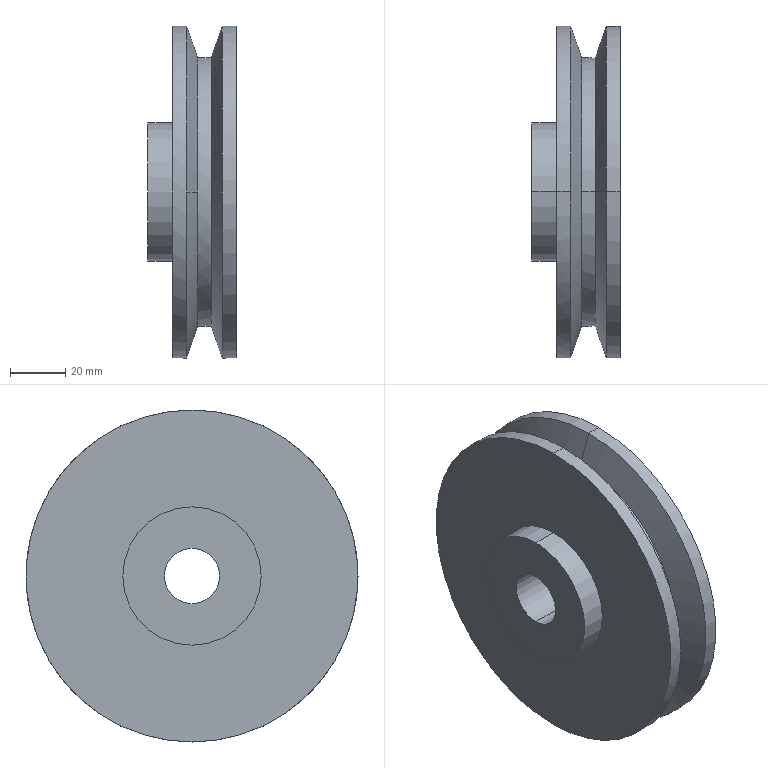Part | SolidWorks | features BaseBody 1, ICE 1 | 1 solid | 17 faces | box 32 x 120 x 120 mm | volume 232249 mm3 | cylinder 10 | cone 4 | plane 3 | commonest cylinder face diameters 120 x4 20 x2 50 x2 97.1 x2
STEP:
#1=CARTESIAN_POINT('',(21.,0.,-10.));
#2=VERTEX_POINT('',#1);
#3=CARTESIAN_POINT('',(21.,0.,10.));
#4=VERTEX_POINT('',#3);
#5=CARTESIAN_POINT('',(21.,0.,0.));
#6=DIRECTION('',(-1.,0.,0.));
#7=DIRECTION('',(0.,0.,1.));
#8=AXIS2_PLACEMENT_3D('',#5,#6,#7);
#9=CIRCLE('',#8,10.);
#10=EDGE_CURVE('',#2,#4,#9,.T.);
#11=ORIENTED_EDGE('',*,*,#10,.F.);
#12=CARTESIAN_POINT('',(-11.,0.,-10.));
#13=VERTEX_POINT('',#12);
#14=CARTESIAN_POINT('',(21.,0.,-10.));
#15=DIRECTION('',(-1.,0.,0.));
#16=VECTOR('',#15,1000.);
#17=LINE('',#14,#16);
#18=EDGE_CURVE('',#2,#13,#17,.T.);
#19=ORIENTED_EDGE('',*,*,#18,.T.);
#20=CARTESIAN_POINT('',(-11.,0.,10.));
#21=VERTEX_POINT('',#20);
#22=CARTESIAN_POINT('',(-11.,0.,0.));
#23=DIRECTION('',(-1.,0.,0.));
#24=DIRECTION('',(0.,0.,1.));
#25=AXIS2_PLACEMENT_3D('',#22,#23,#24);
#26=CIRCLE('',#25,10.);
#27=EDGE_CURVE('',#13,#21,#26,.T.);
#28=ORIENTED_EDGE('',*,*,#27,.T.);
#29=CARTESIAN_POINT('',(21.,0.,10.));
#30=DIRECTION('',(-1.,0.,0.));
#31=VECTOR('',#30,1000.);
#32=LINE('',#29,#31);
#33=EDGE_CURVE('',#4,#21,#32,.T.);
#34=ORIENTED_EDGE('',*,*,#33,.F.);
#35=EDGE_LOOP('',(#11,#19,#28,#34));
#36=FACE_OUTER_BOUND('',#35,.T.);
#37=CARTESIAN_POINT('',(21.,0.,0.));
#38=DIRECTION('',(-1.,0.,0.));
#39=DIRECTION('',(0.,0.,1.));
#40=AXIS2_PLACEMENT_3D('',#37,#38,#39);
#41=CYLINDRICAL_SURFACE('',#40,10.);
#42=ADVANCED_FACE('',(#36),#41,.F.);
#43=CARTESIAN_POINT('',(15.947,0.,-60.));
#44=VERTEX_POINT('',#43);
#45=CARTESIAN_POINT('',(15.947,0.,60.));
#46=VERTEX_POINT('',#45);
#47=CARTESIAN_POINT('',(15.947,0.,0.));
#48=DIRECTION('',(1.,0.,0.));
#49=DIRECTION('',(0.,0.,-1.));
#50=AXIS2_PLACEMENT_3D('',#47,#48,#49);
#51=CIRCLE('',#50,60.);
#52=EDGE_CURVE('',#44,#46,#51,.T.);
#53=ORIENTED_EDGE('',*,*,#52,.T.);
#54=CARTESIAN_POINT('',(21.,0.,60.));
#55=VERTEX_POINT('',#54);
#56=CARTESIAN_POINT('',(0.,0.,60.));
#57=DIRECTION('',(1.,0.,0.));
#58=VECTOR('',#57,1000.);
#59=LINE('',#56,#58);
#60=EDGE_CURVE('',#46,#55,#59,.T.);
#61=ORIENTED_EDGE('',*,*,#60,.T.);
#62=CARTESIAN_POINT('',(21.,0.,-60.));
#63=VERTEX_POINT('',#62);
#64=CARTESIAN_POINT('',(21.,0.,0.));
#65=DIRECTION('',(1.,0.,0.));
#66=DIRECTION('',(0.,0.,-1.));
#67=AXIS2_PLACEMENT_3D('',#64,#65,#66);
#68=CIRCLE('',#67,60.);
#69=EDGE_CURVE('',#63,#55,#68,.T.);
#70=ORIENTED_EDGE('',*,*,#69,.F.);
#71=CARTESIAN_POINT('',(0.,0.,-60.));
#72=DIRECTION('',(1.,0.,0.));
#73=VECTOR('',#72,1000.);
#74=LINE('',#71,#73);
#75=EDGE_CURVE('',#44,#63,#74,.T.);
#76=ORIENTED_EDGE('',*,*,#75,.F.);
#77=EDGE_LOOP('',(#53,#61,#70,#76));
#78=FACE_OUTER_BOUND('',#77,.T.);
#79=CARTESIAN_POINT('',(0.,0.,0.));
#80=DIRECTION('',(1.,0.,0.));
#81=DIRECTION('',(0.,0.,-1.));
#82=AXIS2_PLACEMENT_3D('',#79,#80,#81);
#83=CYLINDRICAL_SURFACE('',#82,60.);
#84=ADVANCED_FACE('',(#78),#83,.T.);
#85=CARTESIAN_POINT('',(12.004,0.,-48.55));
#86=VERTEX_POINT('',#85);
#87=CARTESIAN_POINT('',(12.004,0.,48.55));
#88=VERTEX_POINT('',#87);
#89=CARTESIAN_POINT('',(12.004,0.,0.));
#90=DIRECTION('',(1.,0.,0.));
#91=DIRECTION('',(0.,0.,-1.));
#92=AXIS2_PLACEMENT_3D('',#89,#90,#91);
#93=CIRCLE('',#92,48.55);
#94=EDGE_CURVE('',#86,#88,#93,.T.);
#95=ORIENTED_EDGE('',*,*,#94,.T.);
#96=CARTESIAN_POINT('',(15.947,0.,60.));
#97=DIRECTION('',(0.3256,0.,0.9455));
#98=VECTOR('',#97,1000.);
#99=LINE('',#96,#98);
#100=EDGE_CURVE('',#88,#46,#99,.T.);
#101=ORIENTED_EDGE('',*,*,#100,.T.);
#102=ORIENTED_EDGE('',*,*,#52,.F.);
#103=CARTESIAN_POINT('',(15.947,0.,-60.));
#104=DIRECTION('',(0.3256,0.,-0.9455));
#105=VECTOR('',#104,1000.);
#106=LINE('',#103,#105);
#107=EDGE_CURVE('',#86,#44,#106,.T.);
#108=ORIENTED_EDGE('',*,*,#107,.F.);
#109=EDGE_LOOP('',(#95,#101,#102,#108));
#110=FACE_OUTER_BOUND('',#109,.T.);
#111=CARTESIAN_POINT('',(15.947,0.,0.));
#112=DIRECTION('',(1.,0.,0.));
#113=DIRECTION('',(0.,0.,-1.));
#114=AXIS2_PLACEMENT_3D('',#111,#112,#113);
#115=CONICAL_SURFACE('',#114,60.,1.239);
#116=ADVANCED_FACE('',(#110),#115,.T.);
#117=CARTESIAN_POINT('',(-11.,0.,25.));
#118=VERTEX_POINT('',#117);
#119=CARTESIAN_POINT('',(-11.,0.,-25.));
#120=VERTEX_POINT('',#119);
#121=CARTESIAN_POINT('',(-11.,0.,0.));
#122=DIRECTION('',(-1.,0.,0.));
#123=DIRECTION('',(0.,0.,-1.));
#124=AXIS2_PLACEMENT_3D('',#121,#122,#123);
#125=CIRCLE('',#124,25.);
#126=EDGE_CURVE('',#118,#120,#125,.T.);
#127=ORIENTED_EDGE('',*,*,#126,.F.);
#128=CARTESIAN_POINT('',(-2.,0.,25.));
#129=VERTEX_POINT('',#128);
#130=CARTESIAN_POINT('',(0.,0.,25.));
#131=DIRECTION('',(1.,0.,0.));
#132=VECTOR('',#131,1000.);
#133=LINE('',#130,#132);
#134=EDGE_CURVE('',#118,#129,#133,.T.);
#135=ORIENTED_EDGE('',*,*,#134,.T.);
#136=CARTESIAN_POINT('',(-2.,0.,-25.));
#137=VERTEX_POINT('',#136);
#138=CARTESIAN_POINT('',(-2.,0.,0.));
#139=DIRECTION('',(-1.,0.,0.));
#140=DIRECTION('',(0.,0.,-1.));
#141=AXIS2_PLACEMENT_3D('',#138,#139,#140);
#142=CIRCLE('',#141,25.);
#143=EDGE_CURVE('',#129,#137,#142,.T.);
#144=ORIENTED_EDGE('',*,*,#143,.T.);
#145=CARTESIAN_POINT('',(0.,0.,-25.));
#146=DIRECTION('',(1.,0.,0.));
#147=VECTOR('',#146,1000.);
#148=LINE('',#145,#147);
#149=EDGE_CURVE('',#120,#137,#148,.T.);
#150=ORIENTED_EDGE('',*,*,#149,.F.);
#151=EDGE_LOOP('',(#127,#135,#144,#150));
#152=FACE_OUTER_BOUND('',#151,.T.);
#153=CARTESIAN_POINT('',(0.,0.,0.));
#154=DIRECTION('',(1.,0.,0.));
#155=DIRECTION('',(0.,0.,-1.));
#156=AXIS2_PLACEMENT_3D('',#153,#154,#155);
#157=CYLINDRICAL_SURFACE('',#156,25.);
#158=ADVANCED_FACE('',(#152),#157,.T.);
#159=ORIENTED_EDGE('',*,*,#94,.F.);
#160=CARTESIAN_POINT('',(6.996,0.,-48.55));
#161=VERTEX_POINT('',#160);
#162=CARTESIAN_POINT('',(0.,0.,-48.55));
#163=DIRECTION('',(-1.,0.,0.));
#164=VECTOR('',#163,1000.);
#165=LINE('',#162,#164);
#166=EDGE_CURVE('',#86,#161,#165,.T.);
#167=ORIENTED_EDGE('',*,*,#166,.T.);
#168=CARTESIAN_POINT('',(6.996,48.55,0.));
#169=VERTEX_POINT('',#168);
#170=CARTESIAN_POINT('',(6.996,0.,0.));
#171=DIRECTION('',(1.,0.,0.));
#172=DIRECTION('',(0.,0.,1.));
#173=AXIS2_PLACEMENT_3D('',#170,#171,#172);
#174=CIRCLE('',#173,48.55);
#175=EDGE_CURVE('',#161,#169,#174,.T.);
#176=ORIENTED_EDGE('',*,*,#175,.T.);
#177=CARTESIAN_POINT('',(6.996,0.,48.55));
#178=VERTEX_POINT('',#177);
#179=CARTESIAN_POINT('',(6.996,0.,0.));
#180=DIRECTION('',(1.,0.,0.));
#181=DIRECTION('',(0.,0.,1.));
#182=AXIS2_PLACEMENT_3D('',#179,#180,#181);
#183=CIRCLE('',#182,48.55);
#184=EDGE_CURVE('',#169,#178,#183,.T.);
#185=ORIENTED_EDGE('',*,*,#184,.T.);
#186=CARTESIAN_POINT('',(0.,0.,48.55));
#187=DIRECTION('',(-1.,0.,0.));
#188=VECTOR('',#187,1000.);
#189=LINE('',#186,#188);
#190=EDGE_CURVE('',#88,#178,#189,.T.);
#191=ORIENTED_EDGE('',*,*,#190,.F.);
#192=EDGE_LOOP('',(#159,#167,#176,#185,#191));
#193=FACE_OUTER_BOUND('',#192,.T.);
#194=CARTESIAN_POINT('',(0.,0.,0.));
#195=DIRECTION('',(-1.,0.,0.));
#196=DIRECTION('',(0.,0.,1.));
#197=AXIS2_PLACEMENT_3D('',#194,#195,#196);
#198=CYLINDRICAL_SURFACE('',#197,48.55);
#199=ADVANCED_FACE('',(#193),#198,.T.);
#200=ORIENTED_EDGE('',*,*,#184,.F.);
#201=CARTESIAN_POINT('',(3.053,60.,0.));
#202=VERTEX_POINT('',#201);
#203=CARTESIAN_POINT('',(3.053,60.,0.));
#204=DIRECTION('',(-0.3256,0.9455,0.));
#205=VECTOR('',#204,1000.);
#206=LINE('',#203,#205);
#207=EDGE_CURVE('',#169,#202,#206,.T.);
#208=ORIENTED_EDGE('',*,*,#207,.T.);
#209=CARTESIAN_POINT('',(3.053,0.,60.));
#210=VERTEX_POINT('',#209);
#211=CARTESIAN_POINT('',(3.053,0.,0.));
#212=DIRECTION('',(1.,0.,0.));
#213=DIRECTION('',(0.,0.,1.));
#214=AXIS2_PLACEMENT_3D('',#211,#212,#213);
#215=CIRCLE('',#214,60.);
#216=EDGE_CURVE('',#202,#210,#215,.T.);
#217=ORIENTED_EDGE('',*,*,#216,.T.);
#218=CARTESIAN_POINT('',(3.053,-60.,0.));
#219=VERTEX_POINT('',#218);
#220=CARTESIAN_POINT('',(3.053,0.,0.));
#221=DIRECTION('',(1.,0.,0.));
#222=DIRECTION('',(0.,0.,1.));
#223=AXIS2_PLACEMENT_3D('',#220,#221,#222);
#224=CIRCLE('',#223,60.);
#225=EDGE_CURVE('',#210,#219,#224,.T.);
#226=ORIENTED_EDGE('',*,*,#225,.T.);
#227=CARTESIAN_POINT('',(6.996,-48.55,0.));
#228=VERTEX_POINT('',#227);
#229=CARTESIAN_POINT('',(3.053,-60.,0.));
#230=DIRECTION('',(-0.3256,-0.9455,0.));
#231=VECTOR('',#230,1000.);
#232=LINE('',#229,#231);
#233=EDGE_CURVE('',#228,#219,#232,.T.);
#234=ORIENTED_EDGE('',*,*,#233,.F.);
#235=CARTESIAN_POINT('',(6.996,0.,0.));
#236=DIRECTION('',(1.,0.,0.));
#237=DIRECTION('',(0.,0.,1.));
#238=AXIS2_PLACEMENT_3D('',#235,#236,#237);
#239=CIRCLE('',#238,48.55);
#240=EDGE_CURVE('',#178,#228,#239,.T.);
#241=ORIENTED_EDGE('',*,*,#240,.F.);
#242=EDGE_LOOP('',(#200,#208,#217,#226,#234,#241));
#243=FACE_OUTER_BOUND('',#242,.T.);
#244=CARTESIAN_POINT('',(3.053,0.,0.));
#245=DIRECTION('',(-1.,0.,0.));
#246=DIRECTION('',(0.,-1.,0.));
#247=AXIS2_PLACEMENT_3D('',#244,#245,#246);
#248=CONICAL_SURFACE('',#247,60.,1.239);
#249=ADVANCED_FACE('',(#243),#248,.T.);
#250=CARTESIAN_POINT('',(-2.,0.,60.));
#251=VERTEX_POINT('',#250);
#252=CARTESIAN_POINT('',(-2.,0.,-60.));
#253=VERTEX_POINT('',#252);
#254=CARTESIAN_POINT('',(-2.,0.,0.));
#255=DIRECTION('',(-1.,0.,0.));
#256=DIRECTION('',(0.,0.,-1.));
#257=AXIS2_PLACEMENT_3D('',#254,#255,#256);
#258=CIRCLE('',#257,60.);
#259=EDGE_CURVE('',#251,#253,#258,.T.);
#260=ORIENTED_EDGE('',*,*,#259,.F.);
#261=CARTESIAN_POINT('',(0.,0.,60.));
#262=DIRECTION('',(1.,0.,0.));
#263=VECTOR('',#262,1000.);
#264=LINE('',#261,#263);
#265=EDGE_CURVE('',#251,#210,#264,.T.);
#266=ORIENTED_EDGE('',*,*,#265,.T.);
#267=ORIENTED_EDGE('',*,*,#216,.F.);
#268=CARTESIAN_POINT('',(3.053,0.,-60.));
#269=VERTEX_POINT('',#268);
#270=CARTESIAN_POINT('',(3.053,0.,0.));
#271=DIRECTION('',(1.,0.,0.));
#272=DIRECTION('',(0.,0.,1.));
#273=AXIS2_PLACEMENT_3D('',#270,#271,#272);
#274=CIRCLE('',#273,60.);
#275=EDGE_CURVE('',#269,#202,#274,.T.);
#276=ORIENTED_EDGE('',*,*,#275,.F.);
#277=CARTESIAN_POINT('',(0.,0.,-60.));
#278=DIRECTION('',(1.,0.,0.));
#279=VECTOR('',#278,1000.);
#280=LINE('',#277,#279);
#281=EDGE_CURVE('',#253,#269,#280,.T.);
#282=ORIENTED_EDGE('',*,*,#281,.F.);
#283=EDGE_LOOP('',(#260,#266,#267,#276,#282));
#284=FACE_OUTER_BOUND('',#283,.T.);
#285=CARTESIAN_POINT('',(0.,0.,0.));
#286=DIRECTION('',(1.,0.,0.));
#287=DIRECTION('',(0.,0.,-1.));
#288=AXIS2_PLACEMENT_3D('',#285,#286,#287);
#289=CYLINDRICAL_SURFACE('',#288,60.);
#290=ADVANCED_FACE('',(#284),#289,.T.);
#291=CARTESIAN_POINT('',(21.,0.,0.));
#292=DIRECTION('',(-1.,0.,0.));
#293=DIRECTION('',(0.,0.,1.));
#294=AXIS2_PLACEMENT_3D('',#291,#292,#293);
#295=CIRCLE('',#294,10.);
#296=EDGE_CURVE('',#4,#2,#295,.T.);
#297=ORIENTED_EDGE('',*,*,#296,.T.);
#298=ORIENTED_EDGE('',*,*,#10,.T.);
#299=EDGE_LOOP('',(#297,#298));
#300=FACE_BOUND('',#299,.T.);
#301=ORIENTED_EDGE('',*,*,#69,.T.);
#302=CARTESIAN_POINT('',(21.,0.,0.));
#303=DIRECTION('',(1.,0.,0.));
#304=DIRECTION('',(0.,0.,-1.));
#305=AXIS2_PLACEMENT_3D('',#302,#303,#304);
#306=CIRCLE('',#305,60.);
#307=EDGE_CURVE('',#55,#63,#306,.T.);
#308=ORIENTED_EDGE('',*,*,#307,.T.);
#309=EDGE_LOOP('',(#301,#308));
#310=FACE_OUTER_BOUND('',#309,.T.);
#311=CARTESIAN_POINT('',(21.,60.,0.));
#312=DIRECTION('',(1.,0.,0.));
#313=DIRECTION('',(0.,0.,-1.));
#314=AXIS2_PLACEMENT_3D('',#311,#312,#313);
#315=PLANE('',#314);
#316=ADVANCED_FACE('',(#300,#310),#315,.T.);
#317=ORIENTED_EDGE('',*,*,#60,.F.);
#318=CARTESIAN_POINT('',(15.947,0.,0.));
#319=DIRECTION('',(1.,0.,0.));
#320=DIRECTION('',(0.,0.,-1.));
#321=AXIS2_PLACEMENT_3D('',#318,#319,#320);
#322=CIRCLE('',#321,60.);
#323=EDGE_CURVE('',#46,#44,#322,.T.);
#324=ORIENTED_EDGE('',*,*,#323,.T.);
#325=ORIENTED_EDGE('',*,*,#75,.T.);
#326=ORIENTED_EDGE('',*,*,#307,.F.);
#327=EDGE_LOOP('',(#317,#324,#325,#326));
#328=FACE_OUTER_BOUND('',#327,.T.);
#329=CARTESIAN_POINT('',(0.,0.,0.));
#330=DIRECTION('',(1.,0.,0.));
#331=DIRECTION('',(0.,0.,-1.));
#332=AXIS2_PLACEMENT_3D('',#329,#330,#331);
#333=CYLINDRICAL_SURFACE('',#332,60.);
#334=ADVANCED_FACE('',(#328),#333,.T.);
#335=CARTESIAN_POINT('',(-11.,0.,0.));
#336=DIRECTION('',(-1.,0.,0.));
#337=DIRECTION('',(0.,0.,1.));
#338=AXIS2_PLACEMENT_3D('',#335,#336,#337);
#339=CIRCLE('',#338,10.);
#340=EDGE_CURVE('',#21,#13,#339,.T.);
#341=ORIENTED_EDGE('',*,*,#340,.F.);
#342=ORIENTED_EDGE('',*,*,#27,.F.);
#343=EDGE_LOOP('',(#341,#342));
#344=FACE_BOUND('',#343,.T.);
#345=CARTESIAN_POINT('',(-11.,0.,0.));
#346=DIRECTION('',(-1.,0.,0.));
#347=DIRECTION('',(0.,0.,-1.));
#348=AXIS2_PLACEMENT_3D('',#345,#346,#347);
#349=CIRCLE('',#348,25.);
#350=EDGE_CURVE('',#120,#118,#349,.T.);
#351=ORIENTED_EDGE('',*,*,#350,.T.);
#352=ORIENTED_EDGE('',*,*,#126,.T.);
#353=EDGE_LOOP('',(#351,#352));
#354=FACE_OUTER_BOUND('',#353,.T.);
#355=CARTESIAN_POINT('',(-11.,0.,0.));
#356=DIRECTION('',(-1.,0.,0.));
#357=DIRECTION('',(0.,0.,1.));
#358=AXIS2_PLACEMENT_3D('',#355,#356,#357);
#359=PLANE('',#358);
#360=ADVANCED_FACE('',(#344,#354),#359,.T.);
#361=ORIENTED_EDGE('',*,*,#100,.F.);
#362=CARTESIAN_POINT('',(12.004,0.,0.));
#363=DIRECTION('',(1.,0.,0.));
#364=DIRECTION('',(0.,0.,-1.));
#365=AXIS2_PLACEMENT_3D('',#362,#363,#364);
#366=CIRCLE('',#365,48.55);
#367=EDGE_CURVE('',#88,#86,#366,.T.);
#368=ORIENTED_EDGE('',*,*,#367,.T.);
#369=ORIENTED_EDGE('',*,*,#107,.T.);
#370=ORIENTED_EDGE('',*,*,#323,.F.);
#371=EDGE_LOOP('',(#361,#368,#369,#370));
#372=FACE_OUTER_BOUND('',#371,.T.);
#373=CARTESIAN_POINT('',(15.947,0.,0.));
#374=DIRECTION('',(1.,0.,0.));
#375=DIRECTION('',(0.,0.,-1.));
#376=AXIS2_PLACEMENT_3D('',#373,#374,#375);
#377=CONICAL_SURFACE('',#376,60.,1.239);
#378=ADVANCED_FACE('',(#372),#377,.T.);
#379=ORIENTED_EDGE('',*,*,#134,.F.);
#380=ORIENTED_EDGE('',*,*,#350,.F.);
#381=ORIENTED_EDGE('',*,*,#149,.T.);
#382=CARTESIAN_POINT('',(-2.,0.,0.));
#383=DIRECTION('',(-1.,0.,0.));
#384=DIRECTION('',(0.,0.,-1.));
#385=AXIS2_PLACEMENT_3D('',#382,#383,#384);
#386=CIRCLE('',#385,25.);
#387=EDGE_CURVE('',#137,#129,#386,.T.);
#388=ORIENTED_EDGE('',*,*,#387,.T.);
#389=EDGE_LOOP('',(#379,#380,#381,#388));
#390=FACE_OUTER_BOUND('',#389,.T.);
#391=CARTESIAN_POINT('',(0.,0.,0.));
#392=DIRECTION('',(1.,0.,0.));
#393=DIRECTION('',(0.,0.,-1.));
#394=AXIS2_PLACEMENT_3D('',#391,#392,#393);
#395=CYLINDRICAL_SURFACE('',#394,25.);
#396=ADVANCED_FACE('',(#390),#395,.T.);
#397=ORIENTED_EDGE('',*,*,#166,.F.);
#398=ORIENTED_EDGE('',*,*,#367,.F.);
#399=ORIENTED_EDGE('',*,*,#190,.T.);
#400=ORIENTED_EDGE('',*,*,#240,.T.);
#401=CARTESIAN_POINT('',(6.996,0.,0.));
#402=DIRECTION('',(1.,0.,0.));
#403=DIRECTION('',(0.,0.,1.));
#404=AXIS2_PLACEMENT_3D('',#401,#402,#403);
#405=CIRCLE('',#404,48.55);
#406=EDGE_CURVE('',#228,#161,#405,.T.);
#407=ORIENTED_EDGE('',*,*,#406,.T.);
#408=EDGE_LOOP('',(#397,#398,#399,#400,#407));
#409=FACE_OUTER_BOUND('',#408,.T.);
#410=CARTESIAN_POINT('',(0.,0.,0.));
#411=DIRECTION('',(-1.,0.,0.));
#412=DIRECTION('',(0.,0.,1.));
#413=AXIS2_PLACEMENT_3D('',#410,#411,#412);
#414=CYLINDRICAL_SURFACE('',#413,48.55);
#415=ADVANCED_FACE('',(#409),#414,.T.);
#416=CARTESIAN_POINT('',(-2.,0.,0.));
#417=DIRECTION('',(-1.,0.,0.));
#418=DIRECTION('',(0.,0.,-1.));
#419=AXIS2_PLACEMENT_3D('',#416,#417,#418);
#420=CIRCLE('',#419,60.);
#421=EDGE_CURVE('',#253,#251,#420,.T.);
#422=ORIENTED_EDGE('',*,*,#421,.T.);
#423=ORIENTED_EDGE('',*,*,#259,.T.);
#424=EDGE_LOOP('',(#422,#423));
#425=FACE_OUTER_BOUND('',#424,.T.);
#426=ORIENTED_EDGE('',*,*,#387,.F.);
#427=ORIENTED_EDGE('',*,*,#143,.F.);
#428=EDGE_LOOP('',(#426,#427));
#429=FACE_BOUND('',#428,.T.);
#430=CARTESIAN_POINT('',(-2.,60.,0.));
#431=DIRECTION('',(-1.,0.,0.));
#432=DIRECTION('',(0.,0.,1.));
#433=AXIS2_PLACEMENT_3D('',#430,#431,#432);
#434=PLANE('',#433);
#435=ADVANCED_FACE('',(#425,#429),#434,.T.);
#436=ORIENTED_EDGE('',*,*,#207,.F.);
#437=ORIENTED_EDGE('',*,*,#175,.F.);
#438=ORIENTED_EDGE('',*,*,#406,.F.);
#439=ORIENTED_EDGE('',*,*,#233,.T.);
#440=CARTESIAN_POINT('',(3.053,0.,0.));
#441=DIRECTION('',(1.,0.,0.));
#442=DIRECTION('',(0.,0.,1.));
#443=AXIS2_PLACEMENT_3D('',#440,#441,#442);
#444=CIRCLE('',#443,60.);
#445=EDGE_CURVE('',#219,#269,#444,.T.);
#446=ORIENTED_EDGE('',*,*,#445,.T.);
#447=ORIENTED_EDGE('',*,*,#275,.T.);
#448=EDGE_LOOP('',(#436,#437,#438,#439,#446,#447));
#449=FACE_OUTER_BOUND('',#448,.T.);
#450=CARTESIAN_POINT('',(3.053,0.,0.));
#451=DIRECTION('',(-1.,0.,0.));
#452=DIRECTION('',(0.,-1.,0.));
#453=AXIS2_PLACEMENT_3D('',#450,#451,#452);
#454=CONICAL_SURFACE('',#453,60.,1.239);
#455=ADVANCED_FACE('',(#449),#454,.T.);
#456=ORIENTED_EDGE('',*,*,#265,.F.);
#457=ORIENTED_EDGE('',*,*,#421,.F.);
#458=ORIENTED_EDGE('',*,*,#281,.T.);
#459=ORIENTED_EDGE('',*,*,#445,.F.);
#460=ORIENTED_EDGE('',*,*,#225,.F.);
#461=EDGE_LOOP('',(#456,#457,#458,#459,#460));
#462=FACE_OUTER_BOUND('',#461,.T.);
#463=CARTESIAN_POINT('',(0.,0.,0.));
#464=DIRECTION('',(1.,0.,0.));
#465=DIRECTION('',(0.,0.,-1.));
#466=AXIS2_PLACEMENT_3D('',#463,#464,#465);
#467=CYLINDRICAL_SURFACE('',#466,60.);
#468=ADVANCED_FACE('',(#462),#467,.T.);
#469=ORIENTED_EDGE('',*,*,#18,.F.);
#470=ORIENTED_EDGE('',*,*,#296,.F.);
#471=ORIENTED_EDGE('',*,*,#33,.T.);
#472=ORIENTED_EDGE('',*,*,#340,.T.);
#473=EDGE_LOOP('',(#469,#470,#471,#472));
#474=FACE_OUTER_BOUND('',#473,.T.);
#475=CARTESIAN_POINT('',(21.,0.,0.));
#476=DIRECTION('',(-1.,0.,0.));
#477=DIRECTION('',(0.,0.,1.));
#478=AXIS2_PLACEMENT_3D('',#475,#476,#477);
#479=CYLINDRICAL_SURFACE('',#478,10.);
#480=ADVANCED_FACE('',(#474),#479,.F.);
#481=CLOSED_SHELL('',(#42,#84,#116,#158,#199,#249,#290,#316,#334,#360,#378,#396,#415,#435,#455,#468,#480));
#482=MANIFOLD_SOLID_BREP('',#481);
#483=CARTESIAN_POINT('',(0.,0.,0.));
#484=DIRECTION('',(0.,0.,1.));
#485=DIRECTION('',(1.,0.,0.));
#486=AXIS2_PLACEMENT_3D('',#483,#484,#485);
#487=(LENGTH_UNIT()NAMED_UNIT(*)SI_UNIT(.MILLI.,.METRE.));
#488=UNCERTAINTY_MEASURE_WITH_UNIT(LENGTH_MEASURE(0.00001),#487,'','');
#489=(NAMED_UNIT(*)PLANE_ANGLE_UNIT()SI_UNIT($,.RADIAN.));
#490=(NAMED_UNIT(*)SI_UNIT($,.STERADIAN.)SOLID_ANGLE_UNIT());
#491=(GEOMETRIC_REPRESENTATION_CONTEXT(3)GLOBAL_UNCERTAINTY_ASSIGNED_CONTEXT((#488))GLOBAL_UNIT_ASSIGNED_CONTEXT((#487,#489,#490))REPRESENTATION_CONTEXT('',''));
#492=ADVANCED_BREP_SHAPE_REPRESENTATION('',(#482,#486),#491);